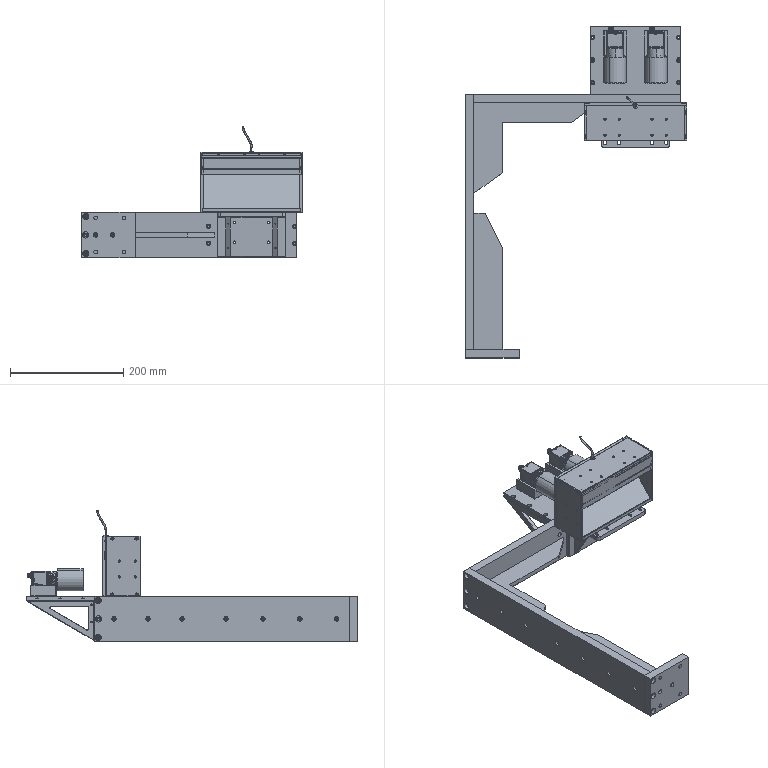Part | SolidWorks | 31 solids | 4494 faces | volume 2173391 mm3 | plane 2316 | cylinder 1364 | cone 462 | spline 346 | torus 6 | commonest cylinder face diameters 0.4 x168 3.3 x100 8 x88 4.5 x80 1.4 x78 2 x60